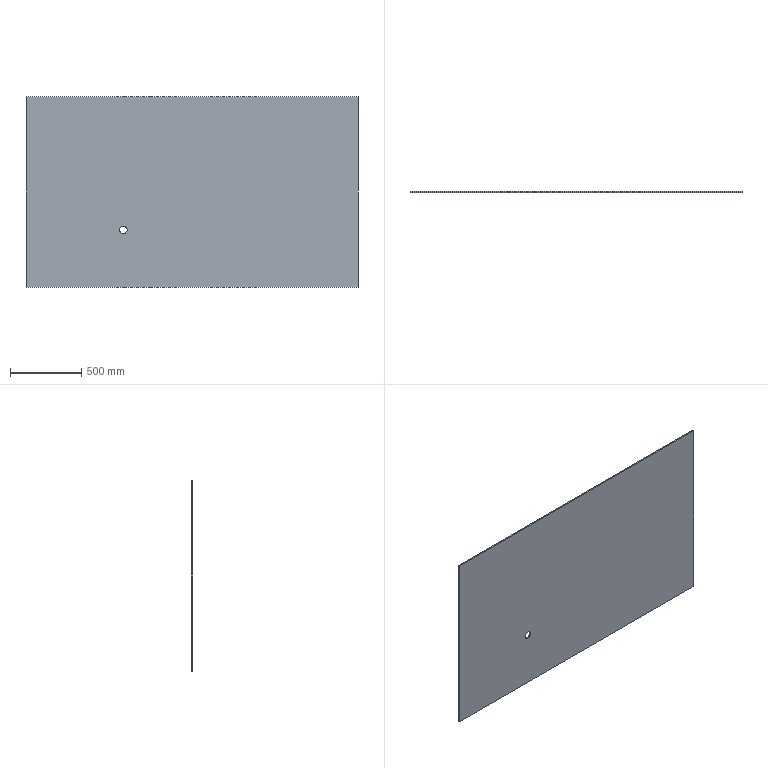Part | SolidWorks | features Extrusion 1 | 1 solid | 8 faces | box 2324 x 8 x 1335 mm | volume 24803330 mm3 | plane 6 | cylinder 2 | commonest cylinder face diameters 52 x2
STEP:
#1=CARTESIAN_POINT('',(-480.,4.,-290.5));
#2=VERTEX_POINT('',#1);
#3=CARTESIAN_POINT('',(-480.,4.,-238.5));
#4=VERTEX_POINT('',#3);
#5=CARTESIAN_POINT('',(-480.,4.,-264.5));
#6=DIRECTION('',(0.,1.,0.));
#7=DIRECTION('',(0.,0.,1.));
#8=AXIS2_PLACEMENT_3D('',#5,#6,#7);
#9=CIRCLE('',#8,26.);
#10=EDGE_CURVE('',#2,#4,#9,.T.);
#11=ORIENTED_EDGE('',*,*,#10,.T.);
#12=CARTESIAN_POINT('',(-480.,-4.,-238.5));
#13=VERTEX_POINT('',#12);
#14=CARTESIAN_POINT('',(-480.,4.,-238.5));
#15=DIRECTION('',(0.,-1.,0.));
#16=VECTOR('',#15,1000.);
#17=LINE('',#14,#16);
#18=EDGE_CURVE('',#4,#13,#17,.T.);
#19=ORIENTED_EDGE('',*,*,#18,.T.);
#20=CARTESIAN_POINT('',(-480.,-4.,-290.5));
#21=VERTEX_POINT('',#20);
#22=CARTESIAN_POINT('',(-480.,-4.,-264.5));
#23=DIRECTION('',(0.,1.,0.));
#24=DIRECTION('',(0.,0.,1.));
#25=AXIS2_PLACEMENT_3D('',#22,#23,#24);
#26=CIRCLE('',#25,26.);
#27=EDGE_CURVE('',#21,#13,#26,.T.);
#28=ORIENTED_EDGE('',*,*,#27,.F.);
#29=CARTESIAN_POINT('',(-480.,4.,-290.5));
#30=DIRECTION('',(0.,-1.,0.));
#31=VECTOR('',#30,1000.);
#32=LINE('',#29,#31);
#33=EDGE_CURVE('',#2,#21,#32,.T.);
#34=ORIENTED_EDGE('',*,*,#33,.F.);
#35=EDGE_LOOP('',(#11,#19,#28,#34));
#36=FACE_OUTER_BOUND('',#35,.T.);
#37=CARTESIAN_POINT('',(-480.,4.,-264.5));
#38=DIRECTION('',(0.,-1.,0.));
#39=DIRECTION('',(0.,0.,-1.));
#40=AXIS2_PLACEMENT_3D('',#37,#38,#39);
#41=CYLINDRICAL_SURFACE('',#40,26.);
#42=ADVANCED_FACE('',(#36),#41,.F.);
#43=CARTESIAN_POINT('',(1162.,4.,667.5));
#44=VERTEX_POINT('',#43);
#45=CARTESIAN_POINT('',(1162.,4.,-667.5));
#46=VERTEX_POINT('',#45);
#47=CARTESIAN_POINT('',(1162.,4.,667.5));
#48=DIRECTION('',(0.,0.,-1.));
#49=VECTOR('',#48,1000.);
#50=LINE('',#47,#49);
#51=EDGE_CURVE('',#44,#46,#50,.T.);
#52=ORIENTED_EDGE('',*,*,#51,.T.);
#53=CARTESIAN_POINT('',(-1162.,4.,-667.5));
#54=VERTEX_POINT('',#53);
#55=CARTESIAN_POINT('',(-1162.,4.,-667.5));
#56=DIRECTION('',(-1.,0.,0.));
#57=VECTOR('',#56,1000.);
#58=LINE('',#55,#57);
#59=EDGE_CURVE('',#46,#54,#58,.T.);
#60=ORIENTED_EDGE('',*,*,#59,.T.);
#61=CARTESIAN_POINT('',(-1162.,4.,667.5));
#62=VERTEX_POINT('',#61);
#63=CARTESIAN_POINT('',(-1162.,4.,667.5));
#64=DIRECTION('',(0.,0.,1.));
#65=VECTOR('',#64,1000.);
#66=LINE('',#63,#65);
#67=EDGE_CURVE('',#54,#62,#66,.T.);
#68=ORIENTED_EDGE('',*,*,#67,.T.);
#69=CARTESIAN_POINT('',(-1162.,4.,667.5));
#70=DIRECTION('',(1.,0.,0.));
#71=VECTOR('',#70,1000.);
#72=LINE('',#69,#71);
#73=EDGE_CURVE('',#62,#44,#72,.T.);
#74=ORIENTED_EDGE('',*,*,#73,.T.);
#75=EDGE_LOOP('',(#52,#60,#68,#74));
#76=FACE_OUTER_BOUND('',#75,.T.);
#77=ORIENTED_EDGE('',*,*,#10,.F.);
#78=CARTESIAN_POINT('',(-480.,4.,-264.5));
#79=DIRECTION('',(0.,1.,0.));
#80=DIRECTION('',(0.,0.,1.));
#81=AXIS2_PLACEMENT_3D('',#78,#79,#80);
#82=CIRCLE('',#81,26.);
#83=EDGE_CURVE('',#4,#2,#82,.T.);
#84=ORIENTED_EDGE('',*,*,#83,.F.);
#85=EDGE_LOOP('',(#77,#84));
#86=FACE_BOUND('',#85,.T.);
#87=CARTESIAN_POINT('',(0.,4.,0.));
#88=DIRECTION('',(0.,-1.,0.));
#89=DIRECTION('',(0.,0.,-1.));
#90=AXIS2_PLACEMENT_3D('',#87,#88,#89);
#91=PLANE('',#90);
#92=ADVANCED_FACE('',(#76,#86),#91,.F.);
#93=CARTESIAN_POINT('',(1162.,-4.,667.5));
#94=VERTEX_POINT('',#93);
#95=CARTESIAN_POINT('',(1162.,-4.,-667.5));
#96=VERTEX_POINT('',#95);
#97=CARTESIAN_POINT('',(1162.,-4.,667.5));
#98=DIRECTION('',(0.,0.,-1.));
#99=VECTOR('',#98,1000.);
#100=LINE('',#97,#99);
#101=EDGE_CURVE('',#94,#96,#100,.T.);
#102=ORIENTED_EDGE('',*,*,#101,.F.);
#103=CARTESIAN_POINT('',(-1162.,-4.,667.5));
#104=VERTEX_POINT('',#103);
#105=CARTESIAN_POINT('',(-1162.,-4.,667.5));
#106=DIRECTION('',(1.,0.,0.));
#107=VECTOR('',#106,1000.);
#108=LINE('',#105,#107);
#109=EDGE_CURVE('',#104,#94,#108,.T.);
#110=ORIENTED_EDGE('',*,*,#109,.F.);
#111=CARTESIAN_POINT('',(-1162.,-4.,-667.5));
#112=VERTEX_POINT('',#111);
#113=CARTESIAN_POINT('',(-1162.,-4.,667.5));
#114=DIRECTION('',(0.,0.,1.));
#115=VECTOR('',#114,1000.);
#116=LINE('',#113,#115);
#117=EDGE_CURVE('',#112,#104,#116,.T.);
#118=ORIENTED_EDGE('',*,*,#117,.F.);
#119=CARTESIAN_POINT('',(-1162.,-4.,-667.5));
#120=DIRECTION('',(-1.,0.,0.));
#121=VECTOR('',#120,1000.);
#122=LINE('',#119,#121);
#123=EDGE_CURVE('',#96,#112,#122,.T.);
#124=ORIENTED_EDGE('',*,*,#123,.F.);
#125=EDGE_LOOP('',(#102,#110,#118,#124));
#126=FACE_OUTER_BOUND('',#125,.T.);
#127=ORIENTED_EDGE('',*,*,#27,.T.);
#128=CARTESIAN_POINT('',(-480.,-4.,-264.5));
#129=DIRECTION('',(0.,1.,0.));
#130=DIRECTION('',(0.,0.,1.));
#131=AXIS2_PLACEMENT_3D('',#128,#129,#130);
#132=CIRCLE('',#131,26.);
#133=EDGE_CURVE('',#13,#21,#132,.T.);
#134=ORIENTED_EDGE('',*,*,#133,.T.);
#135=EDGE_LOOP('',(#127,#134));
#136=FACE_BOUND('',#135,.T.);
#137=CARTESIAN_POINT('',(0.,-4.,0.));
#138=DIRECTION('',(0.,-1.,0.));
#139=DIRECTION('',(0.,0.,-1.));
#140=AXIS2_PLACEMENT_3D('',#137,#138,#139);
#141=PLANE('',#140);
#142=ADVANCED_FACE('',(#126,#136),#141,.T.);
#143=ORIENTED_EDGE('',*,*,#101,.T.);
#144=CARTESIAN_POINT('',(1162.,4.,-667.5));
#145=DIRECTION('',(0.,-1.,0.));
#146=VECTOR('',#145,1000.);
#147=LINE('',#144,#146);
#148=EDGE_CURVE('',#46,#96,#147,.T.);
#149=ORIENTED_EDGE('',*,*,#148,.F.);
#150=ORIENTED_EDGE('',*,*,#51,.F.);
#151=CARTESIAN_POINT('',(1162.,4.,667.5));
#152=DIRECTION('',(0.,-1.,0.));
#153=VECTOR('',#152,1000.);
#154=LINE('',#151,#153);
#155=EDGE_CURVE('',#44,#94,#154,.T.);
#156=ORIENTED_EDGE('',*,*,#155,.T.);
#157=EDGE_LOOP('',(#143,#149,#150,#156));
#158=FACE_OUTER_BOUND('',#157,.T.);
#159=CARTESIAN_POINT('',(1162.,4.,667.5));
#160=DIRECTION('',(-1.,0.,0.));
#161=DIRECTION('',(0.,0.,1.));
#162=AXIS2_PLACEMENT_3D('',#159,#160,#161);
#163=PLANE('',#162);
#164=ADVANCED_FACE('',(#158),#163,.F.);
#165=ORIENTED_EDGE('',*,*,#123,.T.);
#166=CARTESIAN_POINT('',(-1162.,4.,-667.5));
#167=DIRECTION('',(0.,-1.,0.));
#168=VECTOR('',#167,1000.);
#169=LINE('',#166,#168);
#170=EDGE_CURVE('',#54,#112,#169,.T.);
#171=ORIENTED_EDGE('',*,*,#170,.F.);
#172=ORIENTED_EDGE('',*,*,#59,.F.);
#173=ORIENTED_EDGE('',*,*,#148,.T.);
#174=EDGE_LOOP('',(#165,#171,#172,#173));
#175=FACE_OUTER_BOUND('',#174,.T.);
#176=CARTESIAN_POINT('',(-1162.,4.,-667.5));
#177=DIRECTION('',(0.,0.,1.));
#178=DIRECTION('',(1.,0.,0.));
#179=AXIS2_PLACEMENT_3D('',#176,#177,#178);
#180=PLANE('',#179);
#181=ADVANCED_FACE('',(#175),#180,.F.);
#182=ORIENTED_EDGE('',*,*,#117,.T.);
#183=CARTESIAN_POINT('',(-1162.,4.,667.5));
#184=DIRECTION('',(0.,-1.,0.));
#185=VECTOR('',#184,1000.);
#186=LINE('',#183,#185);
#187=EDGE_CURVE('',#62,#104,#186,.T.);
#188=ORIENTED_EDGE('',*,*,#187,.F.);
#189=ORIENTED_EDGE('',*,*,#67,.F.);
#190=ORIENTED_EDGE('',*,*,#170,.T.);
#191=EDGE_LOOP('',(#182,#188,#189,#190));
#192=FACE_OUTER_BOUND('',#191,.T.);
#193=CARTESIAN_POINT('',(-1162.,4.,667.5));
#194=DIRECTION('',(1.,0.,0.));
#195=DIRECTION('',(0.,0.,-1.));
#196=AXIS2_PLACEMENT_3D('',#193,#194,#195);
#197=PLANE('',#196);
#198=ADVANCED_FACE('',(#192),#197,.F.);
#199=ORIENTED_EDGE('',*,*,#109,.T.);
#200=ORIENTED_EDGE('',*,*,#155,.F.);
#201=ORIENTED_EDGE('',*,*,#73,.F.);
#202=ORIENTED_EDGE('',*,*,#187,.T.);
#203=EDGE_LOOP('',(#199,#200,#201,#202));
#204=FACE_OUTER_BOUND('',#203,.T.);
#205=CARTESIAN_POINT('',(-1162.,4.,667.5));
#206=DIRECTION('',(0.,0.,-1.));
#207=DIRECTION('',(-1.,0.,0.));
#208=AXIS2_PLACEMENT_3D('',#205,#206,#207);
#209=PLANE('',#208);
#210=ADVANCED_FACE('',(#204),#209,.F.);
#211=ORIENTED_EDGE('',*,*,#18,.F.);
#212=ORIENTED_EDGE('',*,*,#83,.T.);
#213=ORIENTED_EDGE('',*,*,#33,.T.);
#214=ORIENTED_EDGE('',*,*,#133,.F.);
#215=EDGE_LOOP('',(#211,#212,#213,#214));
#216=FACE_OUTER_BOUND('',#215,.T.);
#217=CARTESIAN_POINT('',(-480.,4.,-264.5));
#218=DIRECTION('',(0.,-1.,0.));
#219=DIRECTION('',(0.,0.,-1.));
#220=AXIS2_PLACEMENT_3D('',#217,#218,#219);
#221=CYLINDRICAL_SURFACE('',#220,26.);
#222=ADVANCED_FACE('',(#216),#221,.F.);
#223=CLOSED_SHELL('',(#42,#92,#142,#164,#181,#198,#210,#222));
#224=MANIFOLD_SOLID_BREP('',#223);
#225=CARTESIAN_POINT('',(0.,0.,0.));
#226=DIRECTION('',(0.,0.,1.));
#227=DIRECTION('',(1.,0.,0.));
#228=AXIS2_PLACEMENT_3D('',#225,#226,#227);
#229=(LENGTH_UNIT()NAMED_UNIT(*)SI_UNIT(.MILLI.,.METRE.));
#230=UNCERTAINTY_MEASURE_WITH_UNIT(LENGTH_MEASURE(0.00001),#229,'','');
#231=(NAMED_UNIT(*)PLANE_ANGLE_UNIT()SI_UNIT($,.RADIAN.));
#232=(NAMED_UNIT(*)SI_UNIT($,.STERADIAN.)SOLID_ANGLE_UNIT());
#233=(GEOMETRIC_REPRESENTATION_CONTEXT(3)GLOBAL_UNCERTAINTY_ASSIGNED_CONTEXT((#230))GLOBAL_UNIT_ASSIGNED_CONTEXT((#229,#231,#232))REPRESENTATION_CONTEXT('',''));
#234=ADVANCED_BREP_SHAPE_REPRESENTATION('',(#224,#228),#233);